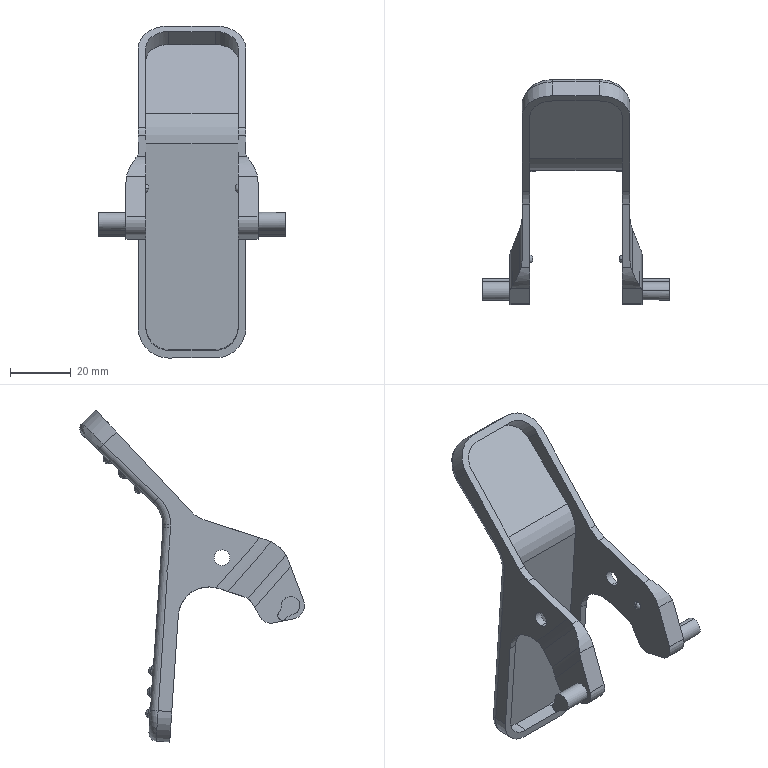Part | SolidWorks | features BaseBody 1 | 1 solid | 142 faces | box 61.4 x 73.898 x 109.12 mm | volume 21040 mm3 | cylinder 69 | plane 32 | torus 21 | sphere 12 | spline 8 | commonest cylinder face diameters 3 x24 20 x14 5 x6 8 x5 5.2 x4 10 x4